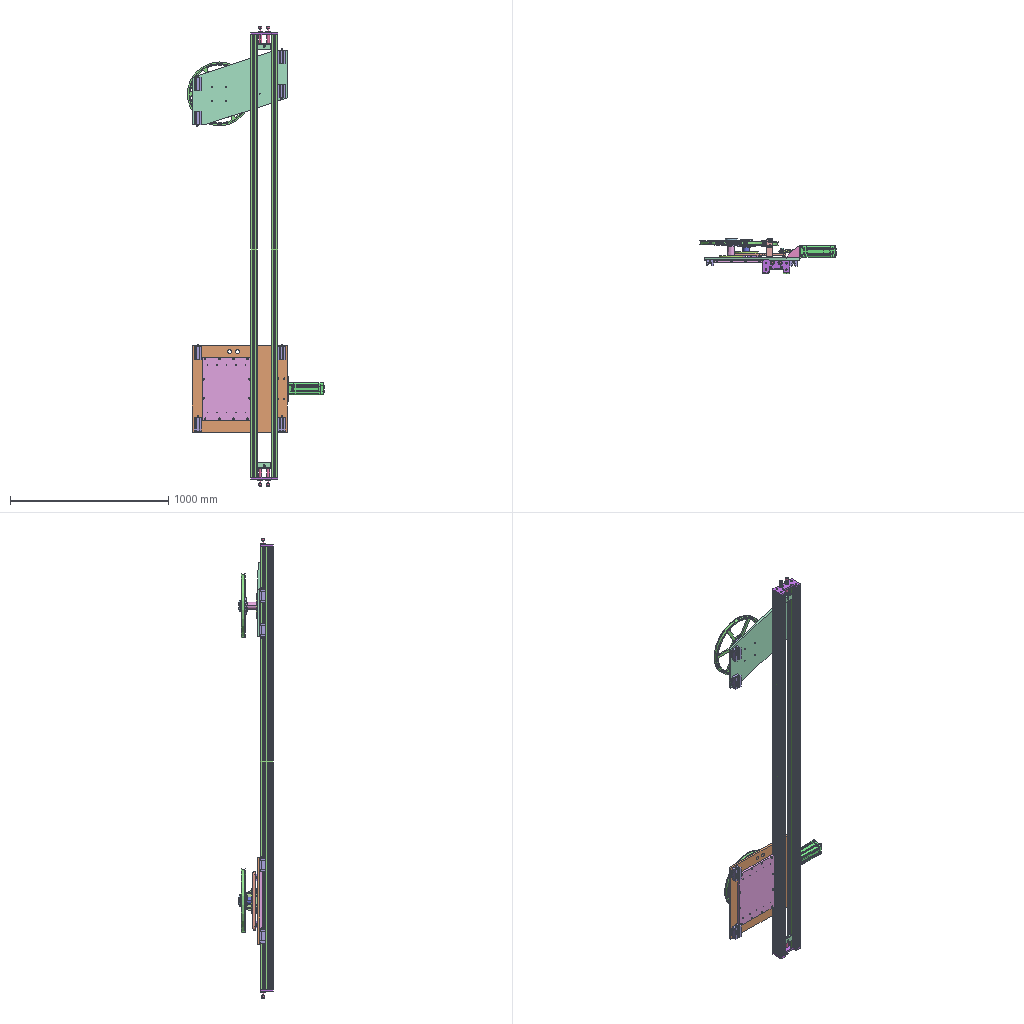Assembly | SolidWorks | 46 different items | 90 placed | box 865 x 218 x 2909 mm
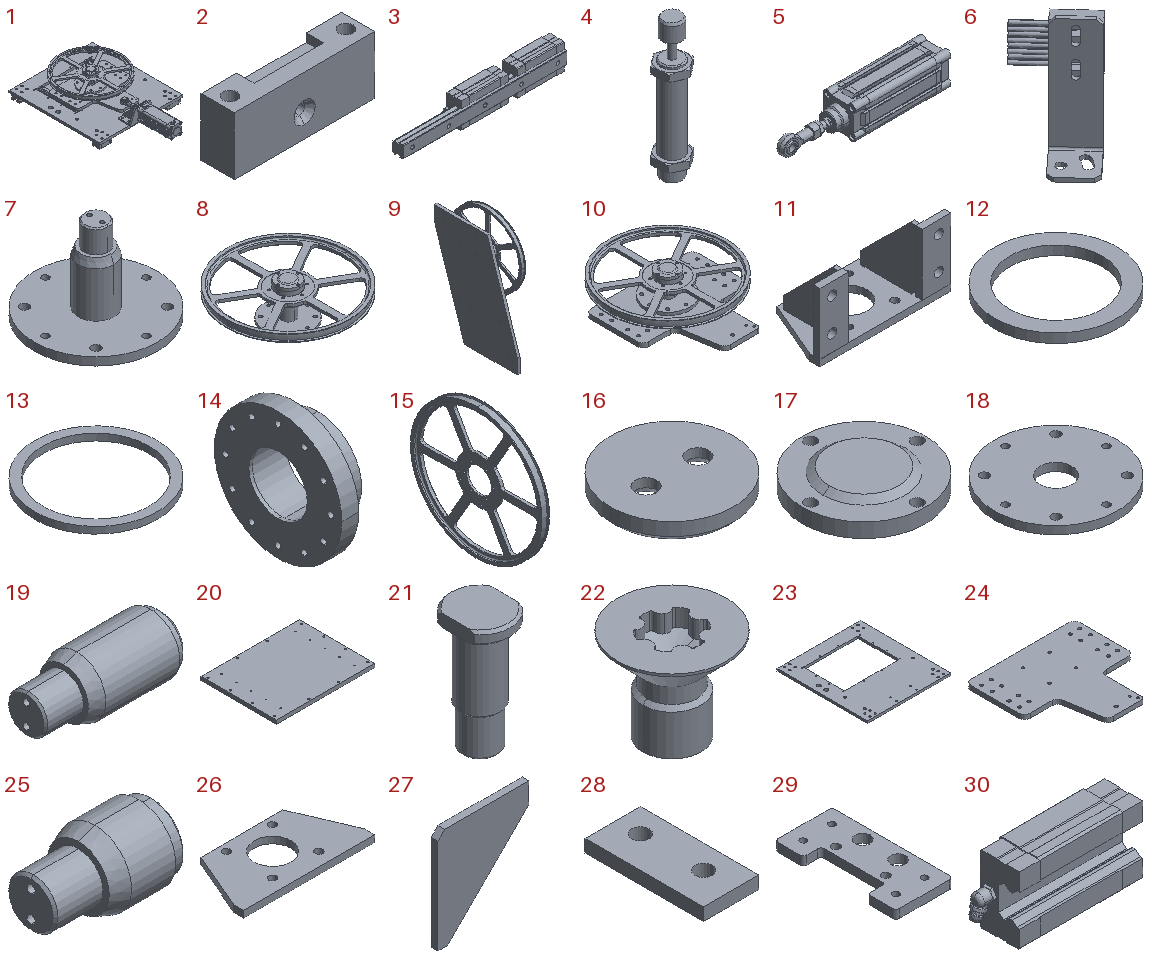Parts list (item | name | quantity | parent item | size | volume | features):
1 | (subassembly) | x1 | - | 554 x 835 x 169.5 mm | 9555082 mm3 | -
2 | (subassembly) | x2 | - | 85 x 20 x 37 mm | 46722 mm3 | -
3 | (subassembly) | x2 | in 1 | 281.473 x 30 x 44 mm | 214734 mm3 | -
4 | (subassembly) | x4 | - | 27.823 x 29.85 x 126 mm | 37470 mm3 | features AEMSimFeature 1
5 | (subassembly) | x1 | in 1 | 364 x 75 x 75 mm | 905739 mm3 | -
6 | (subassembly) | x1 | in 9 | 64.201 x 84.381 x 120 mm | 49700 mm3 | -
7 | (subassembly) | x1 | in 8 | 155 x 155 x 106 mm | 303420 mm3 | -
8 | (subassembly) | x1 | in 9 | 405 x 405 x 120 mm | 1021210 mm3 | -
9 | (subassembly) | x1 | - | 135 x 477.5 x 632.5 mm | 3947731 mm3 | -
10 | (subassembly) | x1 | in 1 | 405 x 452.5 x 105 mm | 2366410 mm3 | -
11 | (subassembly) | x1 | in 1 | 160 x 82.5 x 83 mm | 145011 mm3 | -
12 | - | x2 | in 8, 10 | 40 x 40 x 3 mm | 1649 mm3 | features BaseBody 1
13 | - | x2 | in 8, 10 | 55 x 55 x 3 mm | 1923 mm3 | features BaseBody 1
14 | - | x2 | in 8, 10 | 34 x 109 x 109 mm | 138553 mm3 | features BaseBody 1, CirPattern 1, HoleWzd 1, ICE 1
15 | - | x2 | in 8, 10 | 25 x 405 x 405 mm | 510494 mm3 | features BaseBody 1
16 | - | x2 | in 8, 10 | 38 x 38 x 6 mm | 5863 mm3 | features BaseBody 1
17 | - | x2 | in 8, 10 | 75 x 75 x 13.8 mm | 30557 mm3 | features BaseBody 1, Chamfer 1
18 | - | x2 | in 7, 10 | 155 x 155 x 10 mm | 169991 mm3 | features BaseBody 1, ICE 1
19 | - | x1 | in 7 | 104 x 45 x 45 mm | 133428 mm3 | features BaseBody 1
20 | - | x1 | in 1 | 400 x 308 x 15 mm | 1834801 mm3 | features BaseBody 1
21 | - | x1 | in 1 | 19 x 24 x 48 mm | 9861 mm3 | features BaseBody 1
22 | - | x4 | in 8, 10 | 11.3 x 11.3 x 10 mm | 323.209 mm3 | features BaseBody 1
23 | - | x1 | in 1 | 550 x 600 x 15 mm | 3438854 mm3 | features BaseBody 1, ICE 1
24 | - | x1 | in 10 | 370 x 350 x 15 mm | 1392433 mm3 | features ICE 4, BaseBody 1, Fillet 1
25 | - | x1 | in 10 | 74 x 45 x 45 mm | 86191 mm3 | features BaseBody 1
26 | - | x1 | in 11 | 160 x 82.5 x 8 mm | 73927 mm3 | features BaseBody 1, ICE 1
27 | - | x2 | in 11 | 67 x 5 x 75 mm | 16062 mm3 | features BaseBody 1, Chamfer 1
28 | - | x2 | in 11 | 35 x 75 x 8 mm | 19479 mm3 | features BaseBody 1
29 | - | x2 | - | 80 x 170 x 12 mm | 122295 mm3 | features ICE 2, MoveFace 2, 3DProfileFeature 1, BaseBody 1, Fillet 1, HoleWzd 1
30 | - | x4 | in 3 | 90.473 x 25.7 x 44 mm | 66840 mm3 | features BaseBody 1
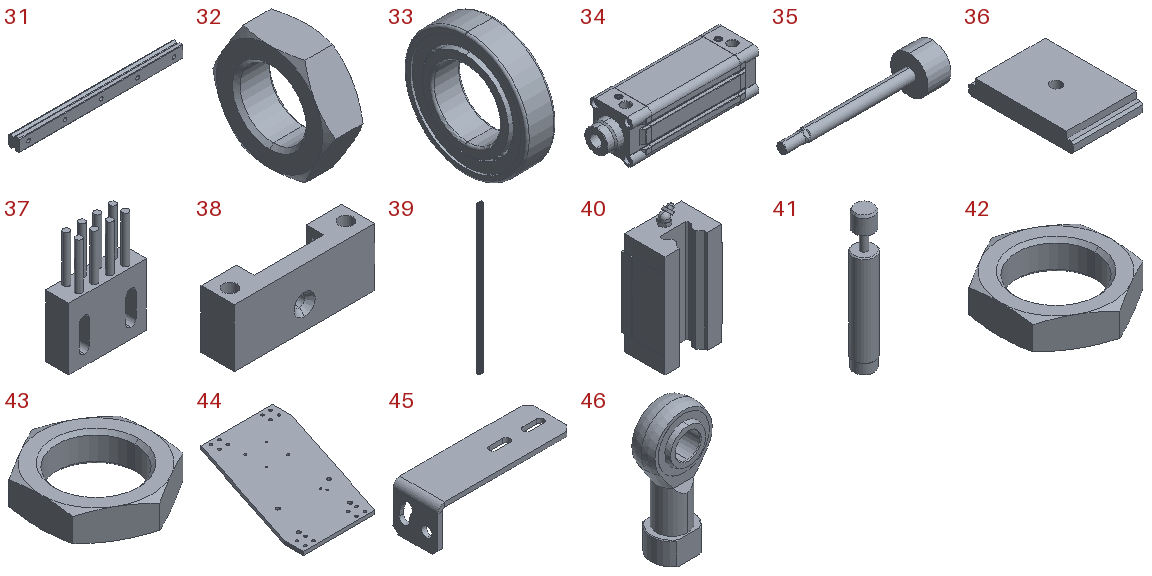31 | - | x2 | in 3 | 270 x 17.5 x 20 mm | 81053 mm3 | features BaseBody 1
32 | - | x1 | in 5 | 8 x 26.558 x 23 mm | 2309 mm3 | features BaseBody 1
33 | - | x4 | in 8, 10 | 13 x 55 x 55 mm | 14054 mm3 | features BaseBody 1
34 | - | x1 | in 5 | 252 x 75 x 75 mm | 699508 mm3 | features BaseBody 1
35 | - | x1 | in 5 | 248.5 x 61.5 x 61.5 mm | 175012 mm3 | features BaseBody 1
36 | - | x2 | in 2 | 32 x 48 x 8 mm | 8228 mm3 | features BaseBody 1, HoleWzd 1
37 | - | x1 | in 6 | 50 x 15 x 70 mm | 26990 mm3 | features BaseBody 1
38 | - | x2 | in 2 | 85 x 20 x 35 mm | 38495 mm3 | features BaseBody 1, HoleWzd 1, MoveFace 1
39 | - | x2 | - | 80 x 40 x 2800 mm | 3366685 mm3 | features BaseBody 1, MoveFace 1
40 | - | x8 | in 1 | 48 x 34.5 x 96 mm | 106215 mm3 | features BaseBody 1
41 | - | x4 | in 4 | 20 x 20 x 126 mm | 33113 mm3 | features MoveFace 2, BaseBody 1
42 | - | x4 | in 4 | 26 x 30 x 7 mm | 2178 mm3 | features BaseBody 1
43 | - | x4 | in 4 | 26 x 30 x 7 mm | 2178 mm3 | features BaseBody 1
44 | - | x1 | in 9 | 470 x 600 x 15 mm | 2876789 mm3 | features BaseBody 1
45 | - | x1 | in 6 | 120 x 40 x 40 mm | 22710 mm3 | features MoveFace 2, BaseBody 1, Chamfer 1, FlatPattern 1, SheetMetal 1, SolidToSheetMetal 1
46 | - | x1 | in 5 | 40 x 22 x 84 mm | 28909 mm3 | features MBimport 1
Mates (type | each side: item.copy, entity, surface, feature):
In the top assembly
Coincident | 41.1 face plane J-WJG12-2050-001 | 41.2 face plane J-WJG12-2050-001
Concentric | 39.1 face cylinder Import1 | 29.1 face cylinder Import1
Concentric | 39.2 face cylinder Import1 | 29.1 face cylinder Import1
Coincident | 39.1 face plane Import1 | 29.1 face plane Import1
Concentric | 29.1 face cylinder Import1 | 38.1 face cylinder Import1 | 2 times
Coincident | 41.3 face plane J-WJG12-2050-001 | 41.4 face plane J-WJG12-2050-001
Coincident | 39.2 face plane Import1 | 29.2 face plane Import1
Concentric | 39.1 face cylinder Import1 | 29.2 face cylinder Import1
Concentric | 39.2 face cylinder Import1 | 29.2 face cylinder Import1
Concentric | 29.2 face cylinder Import1 | 38.2 face cylinder Import1 | 2 times
In subassembly 6
DistanceDim | 37.1 face plane Import1 | 45.1 face plane Convert Entities1
In subassembly 5
Concentric | 35.1 face cylinder Import1 | 46.1 face cylinder F-M16X150U.stp
Coincident | 32.1 face plane Import1 | 46.1 face plane F-M16X150U.stp
Parallel | 34.1 face plane Import1 | 46.1 face plane F-M16X150U.stp
DistanceDim | 32.1 face | 35.1 face plane Import1
In subassembly 4
Concentric | 41.5 face cylinder J-WJG12-2050-001 | 42.1 face cylinder J-WJG12-2050-002
Concentric | 41.5 face cylinder J-WJG12-2050-001 | 43.1 face cylinder J-WJG12-2050-003